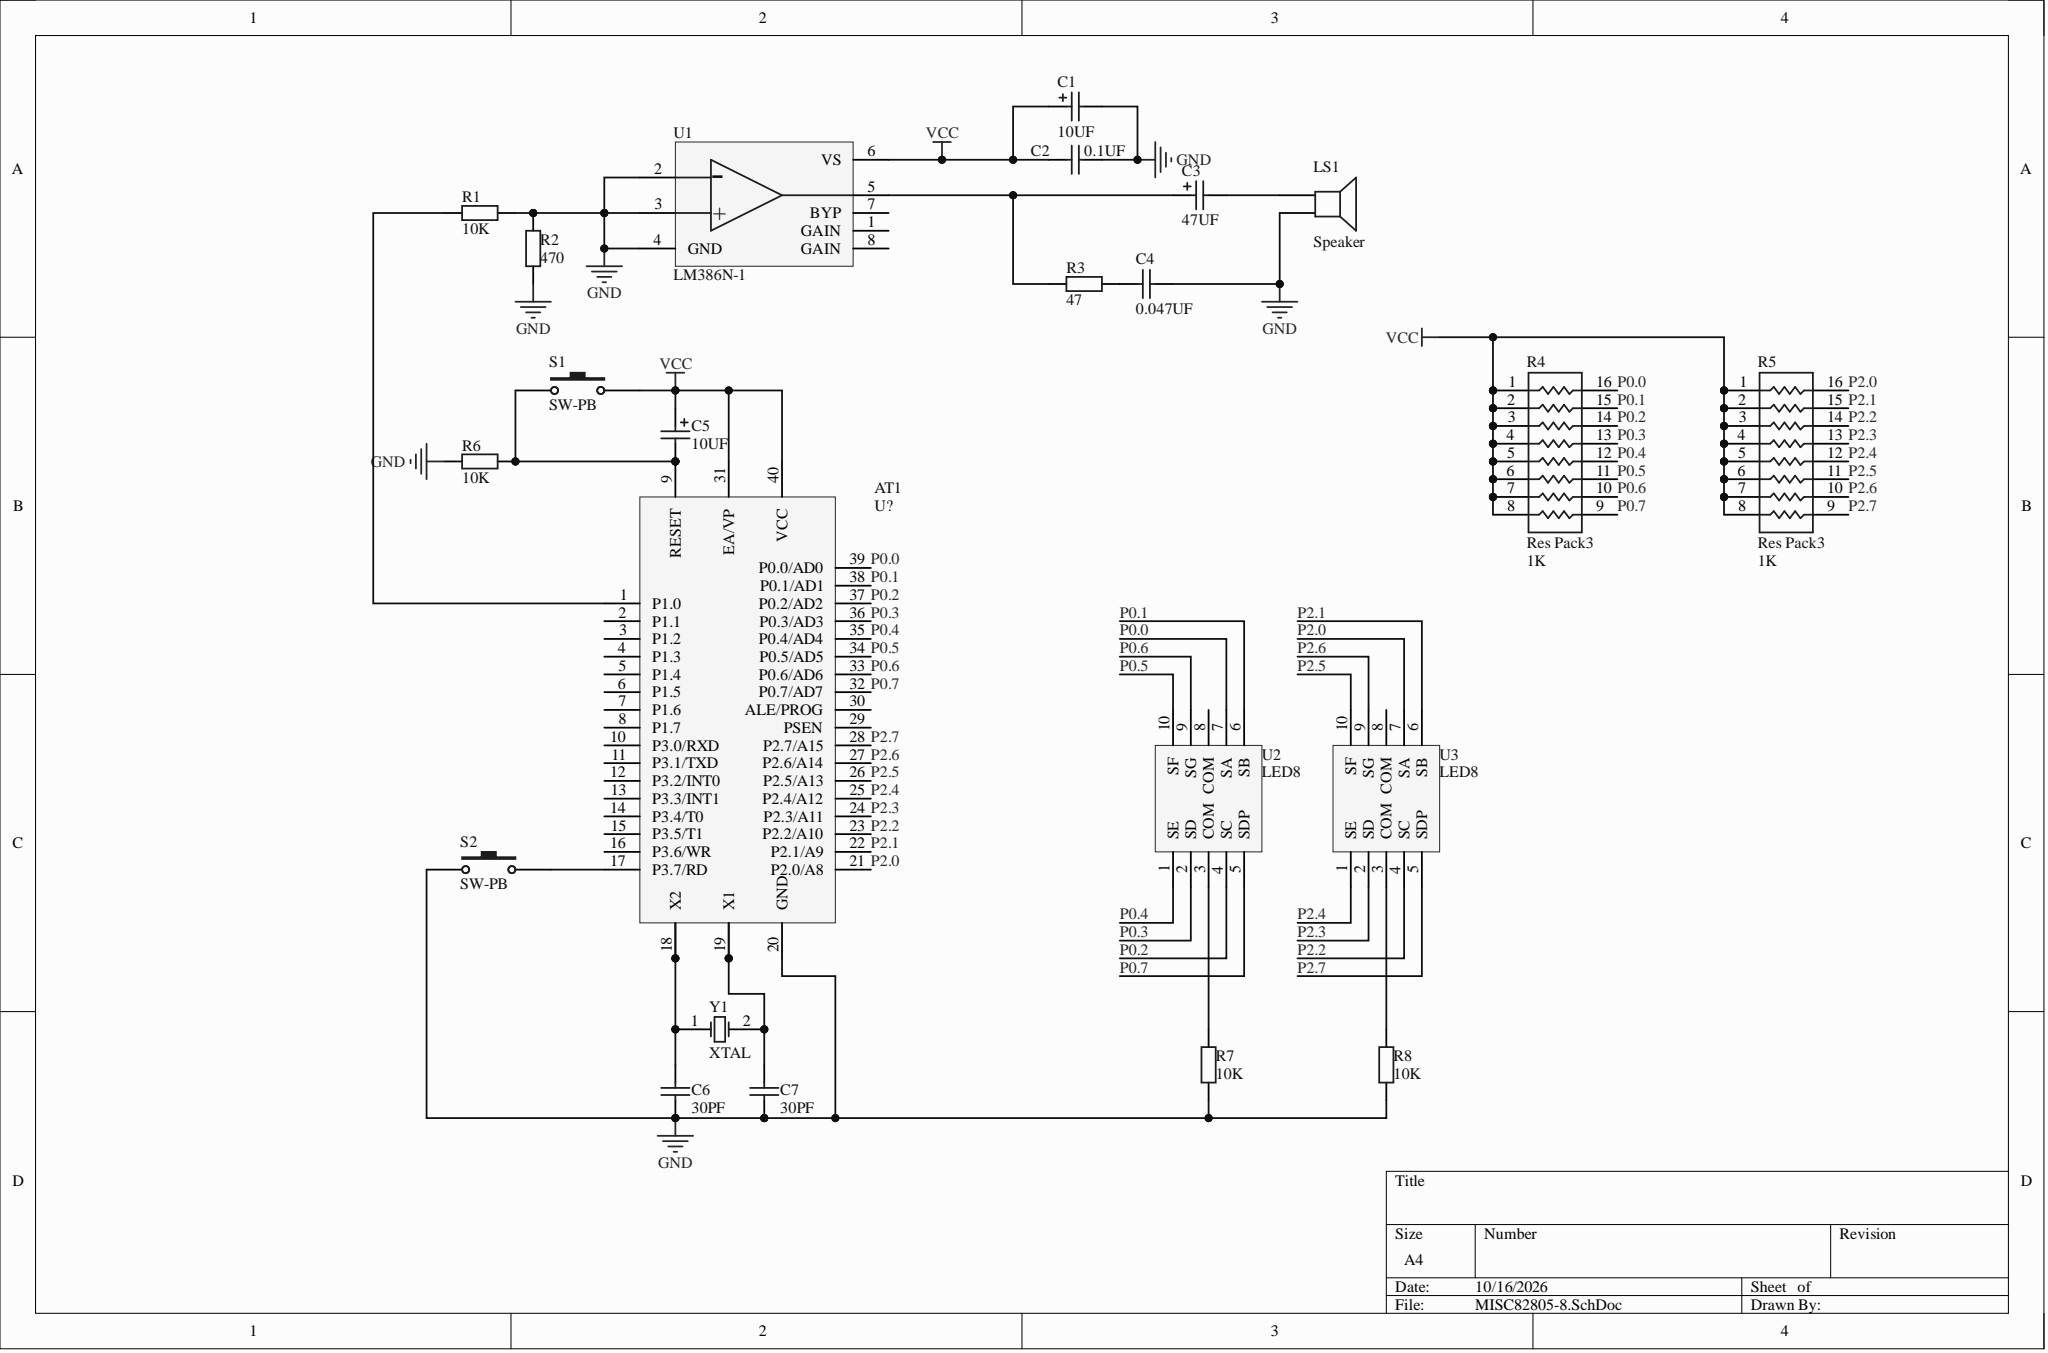Circuit board | Altium Designer | 23 parts | 28 nets
Bill of materials:
Comment,Description,Designator,Footprint,LibRef,Quantity
"U?","","AT1","AT89S52","AT89S52","1"
"10UF","Polarized Capacitor (Axial)","C1, C5","POLAR0.8","Cap Pol2","2"
"0.1UF","Capacitor","C2","RAD-0.3","Cap","1"
"47UF","Polarized Capacitor (Axial)","C3","POLAR0.8","Cap Pol2","1"
"0.047UF","Capacitor","C4","RAD-0.3","Cap","1"
"30PF","Capacitor","C6, C7","RAD-0.3","Cap","2"
"Speaker","Loudspeaker","LS1","PIN2","Speaker","1"
"10K","Resistor","R1, R6, R7, R8","AXIAL-0.4","Res2","4"
"470","Resistor","R2","AXIAL-0.4","Res2","1"
"47","Resistor","R3","AXIAL-0.4","Res2","1"
"Res Pack3","Isolated Resistor Network","R4, R5","SO-16_N","Res Pack3","2"
"SW-PB","Switch","S1, S2","SPST-2","SW-PB","2"
"LM386N-1","","U1","LM386N-1","LM386N-1","1"
"LED8","","U2, U3","LED8","LED8","2"
"XTAL","Crystal Oscillator","Y1","R38","XTAL","1"
Netlist (Protel format):
[
AT1
AT89S52
U?



]
[
C1
POLAR0.8
10UF



]
[
C2
RAD-0.3
0.1UF



]
[
C3
POLAR0.8
47UF



]
[
C4
RAD-0.3
0.047UF



]
[
C5
POLAR0.8
10UF



]
[
C6
RAD-0.3
30PF



]
[
C7
RAD-0.3
30PF



]
[
LS1
PIN2
Speaker



]
[
R1
AXIAL-0.4
10K



]
[
R2
AXIAL-0.4
470



]
[
R3
AXIAL-0.4
47



]
[
R4
SO-16_N
Res Pack3



]
[
R5
SO-16_N
Res Pack3



]
[
R6
AXIAL-0.4
10K



]
[
R7
AXIAL-0.4
10K



]
[
R8
AXIAL-0.4
10K



]
[
S1
SPST-2
SW-PB



]
[
S2
SPST-2
SW-PB



]
[
U1
LM386N-1
LM386N-1



]
[
U2
LED8
LED8



]
[
U3
LED8
LED8



]
[
Y1
R38
XTAL



]
(
VCC
AT1-31
AT1-40
C1-1
C2-1
C5-1
R4-1
R4-2
R4-3
R4-4
R4-5
R4-6
R4-7
R4-8
R5-1
R5-2
R5-3
R5-4
R5-5
R5-6
R5-7
R5-8
S1-2
U1-6
)
(
P2.7
AT1-28
R5-9
U3-5
)
(
P2.6
AT1-27
R5-10
U3-9
)
(
P2.5
AT1-26
R5-11
U3-10
)
(
P2.4
AT1-25
R5-12
U3-1
)
(
P2.3
AT1-24
R5-13
U3-2
)
(
P2.2
AT1-23
R5-14
U3-4
)
(
P2.1
AT1-22
R5-15
U3-6
)
(
P2.0
AT1-21
R5-16
U3-7
)
(
P0.7
AT1-32
R4-9
U2-5
)
(
P0.6
AT1-33
R4-10
U2-9
)
(
P0.5
AT1-34
R4-11
U2-10
)
(
P0.4
AT1-35
R4-12
U2-1
)
(
P0.3
AT1-36
R4-13
U2-2
)
(
P0.2
AT1-37
R4-14
U2-4
)
(
P0.1
AT1-38
R4-15
U2-6
)
(
P0.0
AT1-39
R4-16
U2-7
)
(
NetR8_1
R8-1
U3-3
)
(
NetR7_1
R7-1
U2-3
)
(
NetC4_1
C4-1
R3-2
)
(
NetC3_2
C3-2
LS1-1
)
(
NetC3_1
C3-1
R3-1
U1-5
)
(
NetAT1_19
AT1-19
C7-2
Y1-2
)
(
NetAT1_18
AT1-18
C6-2
Y1-1
)
(
NetAT1_17
AT1-17
S2-2
)
(
NetAT1_9
AT1-9
C5-2
R6-1
S1-1
)
(
NetAT1_1
AT1-1
R1-2
)
(
GND
AT1-20
C1-2
C2-2
C4-2
C6-1
C7-1
LS1-2
R1-1
R2-1
R2-2
R6-2
R7-2
R8-2
S2-1
U1-2
U1-3
U1-4
)